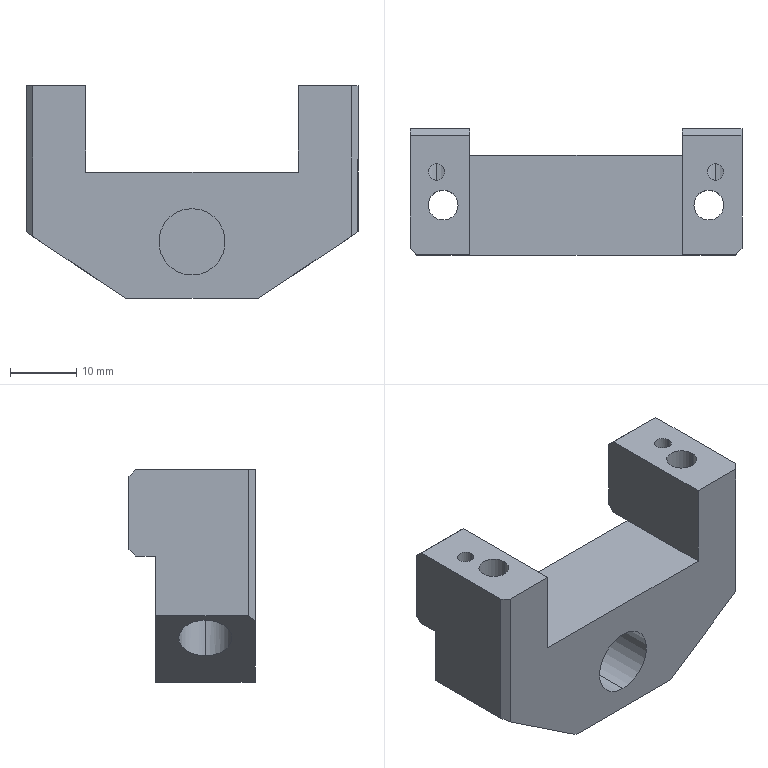Part | SolidWorks | features ICE 5, Chamfer 3, 3DProfileFeature 2, HoleWzd 2, Extrusion 1 | 1 solid | 45 faces | box 50 x 19 x 32 mm | volume 14007 mm3 | plane 27 | cylinder 18 | commonest cylinder face diameters 2.5 x4 4.5 x4 6 x4 8 x4 10 x2
STEP:
#1=CARTESIAN_POINT('',(0.,8.2,-2.5));
#2=VERTEX_POINT('',#1);
#3=CARTESIAN_POINT('',(0.,8.2,-12.5));
#4=VERTEX_POINT('',#3);
#5=CARTESIAN_POINT('',(0.,8.2,-7.5));
#6=DIRECTION('',(0.,-1.,0.));
#7=DIRECTION('',(0.,0.,-1.));
#8=AXIS2_PLACEMENT_3D('',#5,#6,#7);
#9=CIRCLE('',#8,5.);
#10=EDGE_CURVE('',#2,#4,#9,.T.);
#11=ORIENTED_EDGE('',*,*,#10,.F.);
#12=CARTESIAN_POINT('',(0.,0.,-2.5));
#13=VERTEX_POINT('',#12);
#14=CARTESIAN_POINT('',(0.,8.2,-2.5));
#15=DIRECTION('',(0.,-1.,0.));
#16=VECTOR('',#15,1000.);
#17=LINE('',#14,#16);
#18=EDGE_CURVE('',#2,#13,#17,.T.);
#19=ORIENTED_EDGE('',*,*,#18,.T.);
#20=CARTESIAN_POINT('',(0.,0.,-12.5));
#21=VERTEX_POINT('',#20);
#22=CARTESIAN_POINT('',(0.,0.,-7.5));
#23=DIRECTION('',(0.,-1.,0.));
#24=DIRECTION('',(0.,0.,-1.));
#25=AXIS2_PLACEMENT_3D('',#22,#23,#24);
#26=CIRCLE('',#25,5.);
#27=EDGE_CURVE('',#13,#21,#26,.T.);
#28=ORIENTED_EDGE('',*,*,#27,.T.);
#29=CARTESIAN_POINT('',(0.,8.2,-12.5));
#30=DIRECTION('',(0.,-1.,0.));
#31=VECTOR('',#30,1000.);
#32=LINE('',#29,#31);
#33=EDGE_CURVE('',#4,#21,#32,.T.);
#34=ORIENTED_EDGE('',*,*,#33,.F.);
#35=EDGE_LOOP('',(#11,#19,#28,#34));
#36=FACE_OUTER_BOUND('',#35,.T.);
#37=CARTESIAN_POINT('',(0.,8.2,-7.5));
#38=DIRECTION('',(0.,-1.,0.));
#39=DIRECTION('',(0.,0.,-1.));
#40=AXIS2_PLACEMENT_3D('',#37,#38,#39);
#41=CYLINDRICAL_SURFACE('',#40,5.);
#42=ADVANCED_FACE('',(#36),#41,.F.);
#43=CARTESIAN_POINT('',(19.75,12.5,10.727));
#44=VERTEX_POINT('',#43);
#45=CARTESIAN_POINT('',(21.,11.25,11.));
#46=VERTEX_POINT('',#45);
#47=CARTESIAN_POINT('',(19.75,12.5,10.727));
#48=CARTESIAN_POINT('',(19.75,12.335,10.727));
#49=CARTESIAN_POINT('',(19.784,12.169,10.743));
#50=CARTESIAN_POINT('',(19.909,11.868,10.795));
#51=CARTESIAN_POINT('',(20.001,11.731,10.831));
#52=CARTESIAN_POINT('',(20.23,11.502,10.902));
#53=CARTESIAN_POINT('',(20.366,11.41,10.936));
#54=CARTESIAN_POINT('',(20.67,11.283,10.986));
#55=CARTESIAN_POINT('',(20.833,11.25,11.));
#56=CARTESIAN_POINT('',(21.,11.25,11.));
#57=B_SPLINE_CURVE_WITH_KNOTS('',3,(#47,#48,#49,#50,#51,#52,#53,#54,#55,#56),.UNSPECIFIED.,.F.,.F.,(4,2,2,2,4),(0.005929,0.006423,0.006917,0.00741,0.007904),.UNSPECIFIED.);
#58=EDGE_CURVE('',#44,#46,#57,.T.);
#59=ORIENTED_EDGE('',*,*,#58,.F.);
#60=CARTESIAN_POINT('',(19.75,12.5,16.));
#61=VERTEX_POINT('',#60);
#62=CARTESIAN_POINT('',(19.75,12.5,16.));
#63=DIRECTION('',(0.,0.,1.));
#64=VECTOR('',#63,1000.);
#65=LINE('',#62,#64);
#66=EDGE_CURVE('',#44,#61,#65,.T.);
#67=ORIENTED_EDGE('',*,*,#66,.T.);
#68=CARTESIAN_POINT('',(22.25,12.5,16.));
#69=VERTEX_POINT('',#68);
#70=CARTESIAN_POINT('',(21.,12.5,16.));
#71=DIRECTION('',(0.,0.,1.));
#72=DIRECTION('',(1.,0.,0.));
#73=AXIS2_PLACEMENT_3D('',#70,#71,#72);
#74=CIRCLE('',#73,1.25);
#75=EDGE_CURVE('',#61,#69,#74,.T.);
#76=ORIENTED_EDGE('',*,*,#75,.T.);
#77=CARTESIAN_POINT('',(22.25,12.5,10.727));
#78=VERTEX_POINT('',#77);
#79=CARTESIAN_POINT('',(22.25,12.5,16.));
#80=DIRECTION('',(0.,0.,1.));
#81=VECTOR('',#80,1000.);
#82=LINE('',#79,#81);
#83=EDGE_CURVE('',#78,#69,#82,.T.);
#84=ORIENTED_EDGE('',*,*,#83,.F.);
#85=CARTESIAN_POINT('',(21.,11.25,11.));
#86=CARTESIAN_POINT('',(21.084,11.25,11.));
#87=CARTESIAN_POINT('',(21.166,11.258,10.997));
#88=CARTESIAN_POINT('',(21.327,11.291,10.983));
#89=CARTESIAN_POINT('',(21.407,11.315,10.973));
#90=CARTESIAN_POINT('',(21.634,11.41,10.936));
#91=CARTESIAN_POINT('',(21.771,11.503,10.902));
#92=CARTESIAN_POINT('',(21.999,11.731,10.831));
#93=CARTESIAN_POINT('',(22.091,11.869,10.795));
#94=CARTESIAN_POINT('',(22.216,12.169,10.743));
#95=CARTESIAN_POINT('',(22.25,12.335,10.727));
#96=CARTESIAN_POINT('',(22.25,12.5,10.727));
#97=B_SPLINE_CURVE_WITH_KNOTS('',3,(#85,#86,#87,#88,#89,#90,#91,#92,#93,#94,#95,#96),.UNSPECIFIED.,.F.,.F.,(4,2,2,2,2,4),(0.,0.0002472,0.0004944,0.0009888,0.001483,0.001978),.UNSPECIFIED.);
#98=EDGE_CURVE('',#46,#78,#97,.T.);
#99=ORIENTED_EDGE('',*,*,#98,.F.);
#100=EDGE_LOOP('',(#59,#67,#76,#84,#99));
#101=FACE_OUTER_BOUND('',#100,.T.);
#102=CARTESIAN_POINT('',(21.,12.5,16.));
#103=DIRECTION('',(0.,0.,1.));
#104=DIRECTION('',(1.,0.,0.));
#105=AXIS2_PLACEMENT_3D('',#102,#103,#104);
#106=CYLINDRICAL_SURFACE('',#105,1.25);
#107=ADVANCED_FACE('',(#101),#106,.F.);
#108=CARTESIAN_POINT('',(-22.25,12.5,10.727));
#109=VERTEX_POINT('',#108);
#110=CARTESIAN_POINT('',(-21.,11.25,11.));
#111=VERTEX_POINT('',#110);
#112=CARTESIAN_POINT('',(-22.25,12.5,10.727));
#113=CARTESIAN_POINT('',(-22.25,12.335,10.727));
#114=CARTESIAN_POINT('',(-22.216,12.169,10.743));
#115=CARTESIAN_POINT('',(-22.091,11.868,10.795));
#116=CARTESIAN_POINT('',(-21.999,11.731,10.831));
#117=CARTESIAN_POINT('',(-21.77,11.502,10.902));
#118=CARTESIAN_POINT('',(-21.634,11.41,10.936));
#119=CARTESIAN_POINT('',(-21.33,11.283,10.986));
#120=CARTESIAN_POINT('',(-21.167,11.25,11.));
#121=CARTESIAN_POINT('',(-21.,11.25,11.));
#122=B_SPLINE_CURVE_WITH_KNOTS('',3,(#112,#113,#114,#115,#116,#117,#118,#119,#120,#121),.UNSPECIFIED.,.F.,.F.,(4,2,2,2,4),(0.005929,0.006423,0.006917,0.00741,0.007904),.UNSPECIFIED.);
#123=EDGE_CURVE('',#109,#111,#122,.T.);
#124=ORIENTED_EDGE('',*,*,#123,.F.);
#125=CARTESIAN_POINT('',(-22.25,12.5,16.));
#126=VERTEX_POINT('',#125);
#127=CARTESIAN_POINT('',(-22.25,12.5,16.));
#128=DIRECTION('',(0.,0.,1.));
#129=VECTOR('',#128,1000.);
#130=LINE('',#127,#129);
#131=EDGE_CURVE('',#109,#126,#130,.T.);
#132=ORIENTED_EDGE('',*,*,#131,.T.);
#133=CARTESIAN_POINT('',(-19.75,12.5,16.));
#134=VERTEX_POINT('',#133);
#135=CARTESIAN_POINT('',(-21.,12.5,16.));
#136=DIRECTION('',(0.,0.,1.));
#137=DIRECTION('',(1.,0.,0.));
#138=AXIS2_PLACEMENT_3D('',#135,#136,#137);
#139=CIRCLE('',#138,1.25);
#140=EDGE_CURVE('',#126,#134,#139,.T.);
#141=ORIENTED_EDGE('',*,*,#140,.T.);
#142=CARTESIAN_POINT('',(-19.75,12.5,10.727));
#143=VERTEX_POINT('',#142);
#144=CARTESIAN_POINT('',(-19.75,12.5,16.));
#145=DIRECTION('',(0.,0.,1.));
#146=VECTOR('',#145,1000.);
#147=LINE('',#144,#146);
#148=EDGE_CURVE('',#143,#134,#147,.T.);
#149=ORIENTED_EDGE('',*,*,#148,.F.);
#150=CARTESIAN_POINT('',(-21.,11.25,11.));
#151=CARTESIAN_POINT('',(-20.916,11.25,11.));
#152=CARTESIAN_POINT('',(-20.834,11.258,10.997));
#153=CARTESIAN_POINT('',(-20.673,11.291,10.983));
#154=CARTESIAN_POINT('',(-20.593,11.315,10.973));
#155=CARTESIAN_POINT('',(-20.366,11.41,10.936));
#156=CARTESIAN_POINT('',(-20.229,11.503,10.902));
#157=CARTESIAN_POINT('',(-20.001,11.731,10.831));
#158=CARTESIAN_POINT('',(-19.909,11.869,10.795));
#159=CARTESIAN_POINT('',(-19.784,12.169,10.743));
#160=CARTESIAN_POINT('',(-19.75,12.335,10.727));
#161=CARTESIAN_POINT('',(-19.75,12.5,10.727));
#162=B_SPLINE_CURVE_WITH_KNOTS('',3,(#150,#151,#152,#153,#154,#155,#156,#157,#158,#159,#160,#161),.UNSPECIFIED.,.F.,.F.,(4,2,2,2,2,4),(0.,0.0002472,0.0004944,0.0009888,0.001483,0.001978),.UNSPECIFIED.);
#163=EDGE_CURVE('',#111,#143,#162,.T.);
#164=ORIENTED_EDGE('',*,*,#163,.F.);
#165=EDGE_LOOP('',(#124,#132,#141,#149,#164));
#166=FACE_OUTER_BOUND('',#165,.T.);
#167=CARTESIAN_POINT('',(-21.,12.5,16.));
#168=DIRECTION('',(0.,0.,1.));
#169=DIRECTION('',(1.,0.,0.));
#170=AXIS2_PLACEMENT_3D('',#167,#168,#169);
#171=CYLINDRICAL_SURFACE('',#170,1.25);
#172=ADVANCED_FACE('',(#166),#171,.F.);
#173=CARTESIAN_POINT('',(21.,10.8,5.));
#174=VERTEX_POINT('',#173);
#175=CARTESIAN_POINT('',(21.,10.8,11.));
#176=VERTEX_POINT('',#175);
#177=CARTESIAN_POINT('',(21.,10.8,8.));
#178=DIRECTION('',(0.,1.,0.));
#179=DIRECTION('',(0.,0.,1.));
#180=AXIS2_PLACEMENT_3D('',#177,#178,#179);
#181=CIRCLE('',#180,3.);
#182=EDGE_CURVE('',#174,#176,#181,.T.);
#183=ORIENTED_EDGE('',*,*,#182,.F.);
#184=CARTESIAN_POINT('',(21.,19.,5.));
#185=VERTEX_POINT('',#184);
#186=CARTESIAN_POINT('',(21.,10.8,5.));
#187=DIRECTION('',(0.,1.,0.));
#188=VECTOR('',#187,1000.);
#189=LINE('',#186,#188);
#190=EDGE_CURVE('',#174,#185,#189,.T.);
#191=ORIENTED_EDGE('',*,*,#190,.T.);
#192=CARTESIAN_POINT('',(21.,19.,11.));
#193=VERTEX_POINT('',#192);
#194=CARTESIAN_POINT('',(21.,19.,8.));
#195=DIRECTION('',(0.,1.,0.));
#196=DIRECTION('',(0.,0.,1.));
#197=AXIS2_PLACEMENT_3D('',#194,#195,#196);
#198=CIRCLE('',#197,3.);
#199=EDGE_CURVE('',#185,#193,#198,.T.);
#200=ORIENTED_EDGE('',*,*,#199,.T.);
#201=CARTESIAN_POINT('',(21.,13.75,11.));
#202=VERTEX_POINT('',#201);
#203=CARTESIAN_POINT('',(21.,10.8,11.));
#204=DIRECTION('',(0.,1.,0.));
#205=VECTOR('',#204,1000.);
#206=LINE('',#203,#205);
#207=EDGE_CURVE('',#202,#193,#206,.T.);
#208=ORIENTED_EDGE('',*,*,#207,.F.);
#209=CARTESIAN_POINT('',(21.,13.75,11.));
#210=CARTESIAN_POINT('',(20.835,13.75,11.));
#211=CARTESIAN_POINT('',(20.67,13.717,10.986));
#212=CARTESIAN_POINT('',(20.367,13.59,10.936));
#213=CARTESIAN_POINT('',(20.23,13.498,10.902));
#214=CARTESIAN_POINT('',(20.058,13.325,10.849));
#215=CARTESIAN_POINT('',(20.007,13.263,10.831));
#216=CARTESIAN_POINT('',(19.917,13.129,10.798));
#217=CARTESIAN_POINT('',(19.878,13.056,10.782));
#218=CARTESIAN_POINT('',(19.815,12.906,10.756));
#219=CARTESIAN_POINT('',(19.791,12.828,10.746));
#220=CARTESIAN_POINT('',(19.758,12.666,10.731));
#221=CARTESIAN_POINT('',(19.75,12.582,10.727));
#222=CARTESIAN_POINT('',(19.75,12.5,10.727));
#223=B_SPLINE_CURVE_WITH_KNOTS('',3,(#209,#210,#211,#212,#213,#214,#215,#216,#217,#218,#219,#220,#221,#222),.UNSPECIFIED.,.F.,.F.,(4,2,2,2,2,2,4),(0.003954,0.004448,0.004941,0.005188,0.005435,0.005682,0.005929),.UNSPECIFIED.);
#224=EDGE_CURVE('',#202,#44,#223,.T.);
#225=ORIENTED_EDGE('',*,*,#224,.T.);
#226=ORIENTED_EDGE('',*,*,#58,.T.);
#227=CARTESIAN_POINT('',(21.,10.8,11.));
#228=DIRECTION('',(0.,1.,0.));
#229=VECTOR('',#228,1000.);
#230=LINE('',#227,#229);
#231=EDGE_CURVE('',#176,#46,#230,.T.);
#232=ORIENTED_EDGE('',*,*,#231,.F.);
#233=EDGE_LOOP('',(#183,#191,#200,#208,#225,#226,#232));
#234=FACE_OUTER_BOUND('',#233,.T.);
#235=CARTESIAN_POINT('',(21.,10.8,8.));
#236=DIRECTION('',(0.,1.,0.));
#237=DIRECTION('',(0.,0.,1.));
#238=AXIS2_PLACEMENT_3D('',#235,#236,#237);
#239=CYLINDRICAL_SURFACE('',#238,3.);
#240=ADVANCED_FACE('',(#234),#239,.F.);
#241=CARTESIAN_POINT('',(-21.,10.8,5.));
#242=VERTEX_POINT('',#241);
#243=CARTESIAN_POINT('',(-21.,10.8,11.));
#244=VERTEX_POINT('',#243);
#245=CARTESIAN_POINT('',(-21.,10.8,8.));
#246=DIRECTION('',(0.,1.,0.));
#247=DIRECTION('',(0.,0.,1.));
#248=AXIS2_PLACEMENT_3D('',#245,#246,#247);
#249=CIRCLE('',#248,3.);
#250=EDGE_CURVE('',#242,#244,#249,.T.);
#251=ORIENTED_EDGE('',*,*,#250,.F.);
#252=CARTESIAN_POINT('',(-21.,19.,5.));
#253=VERTEX_POINT('',#252);
#254=CARTESIAN_POINT('',(-21.,10.8,5.));
#255=DIRECTION('',(0.,1.,0.));
#256=VECTOR('',#255,1000.);
#257=LINE('',#254,#256);
#258=EDGE_CURVE('',#242,#253,#257,.T.);
#259=ORIENTED_EDGE('',*,*,#258,.T.);
#260=CARTESIAN_POINT('',(-21.,19.,11.));
#261=VERTEX_POINT('',#260);
#262=CARTESIAN_POINT('',(-21.,19.,8.));
#263=DIRECTION('',(0.,1.,0.));
#264=DIRECTION('',(0.,0.,1.));
#265=AXIS2_PLACEMENT_3D('',#262,#263,#264);
#266=CIRCLE('',#265,3.);
#267=EDGE_CURVE('',#253,#261,#266,.T.);
#268=ORIENTED_EDGE('',*,*,#267,.T.);
#269=CARTESIAN_POINT('',(-21.,13.75,11.));
#270=VERTEX_POINT('',#269);
#271=CARTESIAN_POINT('',(-21.,10.8,11.));
#272=DIRECTION('',(0.,1.,0.));
#273=VECTOR('',#272,1000.);
#274=LINE('',#271,#273);
#275=EDGE_CURVE('',#270,#261,#274,.T.);
#276=ORIENTED_EDGE('',*,*,#275,.F.);
#277=CARTESIAN_POINT('',(-21.,13.75,11.));
#278=CARTESIAN_POINT('',(-21.165,13.75,11.));
#279=CARTESIAN_POINT('',(-21.33,13.717,10.986));
#280=CARTESIAN_POINT('',(-21.633,13.59,10.936));
#281=CARTESIAN_POINT('',(-21.77,13.498,10.902));
#282=CARTESIAN_POINT('',(-21.942,13.325,10.849));
#283=CARTESIAN_POINT('',(-21.993,13.263,10.831));
#284=CARTESIAN_POINT('',(-22.083,13.129,10.798));
#285=CARTESIAN_POINT('',(-22.122,13.056,10.782));
#286=CARTESIAN_POINT('',(-22.185,12.906,10.756));
#287=CARTESIAN_POINT('',(-22.209,12.828,10.746));
#288=CARTESIAN_POINT('',(-22.242,12.666,10.731));
#289=CARTESIAN_POINT('',(-22.25,12.582,10.727));
#290=CARTESIAN_POINT('',(-22.25,12.5,10.727));
#291=B_SPLINE_CURVE_WITH_KNOTS('',3,(#277,#278,#279,#280,#281,#282,#283,#284,#285,#286,#287,#288,#289,#290),.UNSPECIFIED.,.F.,.F.,(4,2,2,2,2,2,4),(0.003954,0.004448,0.004941,0.005188,0.005435,0.005682,0.005929),.UNSPECIFIED.);
#292=EDGE_CURVE('',#270,#109,#291,.T.);
#293=ORIENTED_EDGE('',*,*,#292,.T.);
#294=ORIENTED_EDGE('',*,*,#123,.T.);
#295=CARTESIAN_POINT('',(-21.,10.8,11.));
#296=DIRECTION('',(0.,1.,0.));
#297=VECTOR('',#296,1000.);
#298=LINE('',#295,#297);
#299=EDGE_CURVE('',#244,#111,#298,.T.);
#300=ORIENTED_EDGE('',*,*,#299,.F.);
#301=EDGE_LOOP('',(#251,#259,#268,#276,#293,#294,#300));
#302=FACE_OUTER_BOUND('',#301,.T.);
#303=CARTESIAN_POINT('',(-21.,10.8,8.));
#304=DIRECTION('',(0.,1.,0.));
#305=DIRECTION('',(0.,0.,1.));
#306=AXIS2_PLACEMENT_3D('',#303,#304,#305);
#307=CYLINDRICAL_SURFACE('',#306,3.);
#308=ADVANCED_FACE('',(#302),#307,.F.);
#309=CARTESIAN_POINT('',(-16.,7.5,-3.));
#310=VERTEX_POINT('',#309);
#311=CARTESIAN_POINT('',(-24.,7.5,-3.));
#312=VERTEX_POINT('',#311);
#313=CARTESIAN_POINT('',(-20.,7.5,-3.));
#314=DIRECTION('',(0.,0.,-1.));
#315=DIRECTION('',(-1.,0.,0.));
#316=AXIS2_PLACEMENT_3D('',#313,#314,#315);
#317=CIRCLE('',#316,4.);
#318=EDGE_CURVE('',#310,#312,#317,.T.);
#319=ORIENTED_EDGE('',*,*,#318,.F.);
#320=CARTESIAN_POINT('',(-16.,7.5,-12.));
#321=VERTEX_POINT('',#320);
#322=CARTESIAN_POINT('',(-16.,7.5,-3.));
#323=DIRECTION('',(0.,0.,-1.));
#324=VECTOR('',#323,1000.);
#325=LINE('',#322,#324);
#326=EDGE_CURVE('',#310,#321,#325,.T.);
#327=ORIENTED_EDGE('',*,*,#326,.T.);
#328=CARTESIAN_POINT('',(-24.,7.5,-6.667));
#329=VERTEX_POINT('',#328);
#330=CARTESIAN_POINT('',(-16.,7.5,-12.));
#331=CARTESIAN_POINT('',(-16.,-0.5,-12.));
#332=CARTESIAN_POINT('',(-24.,-0.5,-6.667));
#333=CARTESIAN_POINT('',(-24.,7.5,-6.667));
#334=(BOUNDED_CURVE()B_SPLINE_CURVE(3,(#330,#331,#332,#333),.UNSPECIFIED.,.F.,.F.)B_SPLINE_CURVE_WITH_KNOTS((4,4),(0.,3.142),.UNSPECIFIED.)CURVE()GEOMETRIC_REPRESENTATION_ITEM()RATIONAL_B_SPLINE_CURVE((1.,0.3333,0.3333,1.))REPRESENTATION_ITEM(''));
#335=EDGE_CURVE('',#321,#329,#334,.T.);
#336=ORIENTED_EDGE('',*,*,#335,.T.);
#337=CARTESIAN_POINT('',(-24.,7.5,-3.));
#338=DIRECTION('',(0.,0.,-1.));
#339=VECTOR('',#338,1000.);
#340=LINE('',#337,#339);
#341=EDGE_CURVE('',#312,#329,#340,.T.);
#342=ORIENTED_EDGE('',*,*,#341,.F.);
#343=EDGE_LOOP('',(#319,#327,#336,#342));
#344=FACE_OUTER_BOUND('',#343,.T.);
#345=CARTESIAN_POINT('',(-20.,7.5,-3.));
#346=DIRECTION('',(0.,0.,-1.));
#347=DIRECTION('',(-1.,0.,0.));
#348=AXIS2_PLACEMENT_3D('',#345,#346,#347);
#349=CYLINDRICAL_SURFACE('',#348,4.);
#350=ADVANCED_FACE('',(#344),#349,.F.);
#351=CARTESIAN_POINT('',(24.,7.5,-3.));
#352=VERTEX_POINT('',#351);
#353=CARTESIAN_POINT('',(16.,7.5,-3.));
#354=VERTEX_POINT('',#353);
#355=CARTESIAN_POINT('',(20.,7.5,-3.));
#356=DIRECTION('',(0.,0.,-1.));
#357=DIRECTION('',(-1.,0.,0.));
#358=AXIS2_PLACEMENT_3D('',#355,#356,#357);
#359=CIRCLE('',#358,4.);
#360=EDGE_CURVE('',#352,#354,#359,.T.);
#361=ORIENTED_EDGE('',*,*,#360,.F.);
#362=CARTESIAN_POINT('',(24.,7.5,-6.667));
#363=VERTEX_POINT('',#362);
#364=CARTESIAN_POINT('',(24.,7.5,-3.));
#365=DIRECTION('',(0.,0.,-1.));
#366=VECTOR('',#365,1000.);
#367=LINE('',#364,#366);
#368=EDGE_CURVE('',#352,#363,#367,.T.);
#369=ORIENTED_EDGE('',*,*,#368,.T.);
#370=CARTESIAN_POINT('',(16.,7.5,-12.));
#371=VERTEX_POINT('',#370);
#372=CARTESIAN_POINT('',(24.,7.5,-6.667));
#373=CARTESIAN_POINT('',(24.,-0.5,-6.667));
#374=CARTESIAN_POINT('',(16.,-0.5,-12.));
#375=CARTESIAN_POINT('',(16.,7.5,-12.));
#376=(BOUNDED_CURVE()B_SPLINE_CURVE(3,(#372,#373,#374,#375),.UNSPECIFIED.,.F.,.F.)B_SPLINE_CURVE_WITH_KNOTS((4,4),(3.142,6.283),.UNSPECIFIED.)CURVE()GEOMETRIC_REPRESENTATION_ITEM()RATIONAL_B_SPLINE_CURVE((1.,0.3333,0.3333,1.))REPRESENTATION_ITEM(''));
#377=EDGE_CURVE('',#363,#371,#376,.T.);
#378=ORIENTED_EDGE('',*,*,#377,.T.);
#379=CARTESIAN_POINT('',(16.,7.5,-3.));
#380=DIRECTION('',(0.,0.,-1.));
#381=VECTOR('',#380,1000.);
#382=LINE('',#379,#381);
#383=EDGE_CURVE('',#354,#371,#382,.T.);
#384=ORIENTED_EDGE('',*,*,#383,.F.);
#385=EDGE_LOOP('',(#361,#369,#378,#384));
#386=FACE_OUTER_BOUND('',#385,.T.);
#387=CARTESIAN_POINT('',(20.,7.5,-3.));
#388=DIRECTION('',(0.,0.,-1.));
#389=DIRECTION('',(-1.,0.,0.));
#390=AXIS2_PLACEMENT_3D('',#387,#388,#389);
#391=CYLINDRICAL_SURFACE('',#390,4.);
#392=ADVANCED_FACE('',(#386),#391,.F.);
#393=CARTESIAN_POINT('',(22.25,7.5,16.));
#394=VERTEX_POINT('',#393);
#395=CARTESIAN_POINT('',(17.75,7.5,16.));
#396=VERTEX_POINT('',#395);
#397=CARTESIAN_POINT('',(20.,7.5,16.));
#398=DIRECTION('',(0.,0.,-1.));
#399=DIRECTION('',(-1.,0.,0.));
#400=AXIS2_PLACEMENT_3D('',#397,#398,#399);
#401=CIRCLE('',#400,2.25);
#402=EDGE_CURVE('',#394,#396,#401,.T.);
#403=ORIENTED_EDGE('',*,*,#402,.F.);
#404=CARTESIAN_POINT('',(22.25,7.5,-3.));
#405=VERTEX_POINT('',#404);
#406=CARTESIAN_POINT('',(22.25,7.5,20.));
#407=DIRECTION('',(0.,0.,-1.));
#408=VECTOR('',#407,1000.);
#409=LINE('',#406,#408);
#410=EDGE_CURVE('',#394,#405,#409,.T.);
#411=ORIENTED_EDGE('',*,*,#410,.T.);
#412=CARTESIAN_POINT('',(17.75,7.5,-3.));
#413=VERTEX_POINT('',#412);
#414=CARTESIAN_POINT('',(20.,7.5,-3.));
#415=DIRECTION('',(0.,0.,1.));
#416=DIRECTION('',(-1.,0.,0.));
#417=AXIS2_PLACEMENT_3D('',#414,#415,#416);
#418=CIRCLE('',#417,2.25);
#419=EDGE_CURVE('',#413,#405,#418,.T.);
#420=ORIENTED_EDGE('',*,*,#419,.F.);
#421=CARTESIAN_POINT('',(17.75,7.5,20.));
#422=DIRECTION('',(0.,0.,-1.));
#423=VECTOR('',#422,1000.);
#424=LINE('',#421,#423);
#425=EDGE_CURVE('',#396,#413,#424,.T.);
#426=ORIENTED_EDGE('',*,*,#425,.F.);
#427=EDGE_LOOP('',(#403,#411,#420,#426));
#428=FACE_OUTER_BOUND('',#427,.T.);
#429=CARTESIAN_POINT('',(20.,7.5,20.));
#430=DIRECTION('',(0.,0.,-1.));
#431=DIRECTION('',(-1.,0.,0.));
#432=AXIS2_PLACEMENT_3D('',#429,#430,#431);
#433=CYLINDRICAL_SURFACE('',#432,2.25);
#434=ADVANCED_FACE('',(#428),#433,.F.);
#435=CARTESIAN_POINT('',(-17.75,7.5,16.));
#436=VERTEX_POINT('',#435);
#437=CARTESIAN_POINT('',(-22.25,7.5,16.));
#438=VERTEX_POINT('',#437);
#439=CARTESIAN_POINT('',(-20.,7.5,16.));
#440=DIRECTION('',(0.,0.,-1.));
#441=DIRECTION('',(-1.,0.,0.));
#442=AXIS2_PLACEMENT_3D('',#439,#440,#441);
#443=CIRCLE('',#442,2.25);
#444=EDGE_CURVE('',#436,#438,#443,.T.);
#445=ORIENTED_EDGE('',*,*,#444,.F.);
#446=CARTESIAN_POINT('',(-17.75,7.5,-3.));
#447=VERTEX_POINT('',#446);
#448=CARTESIAN_POINT('',(-17.75,7.5,20.));
#449=DIRECTION('',(0.,0.,-1.));
#450=VECTOR('',#449,1000.);
#451=LINE('',#448,#450);
#452=EDGE_CURVE('',#436,#447,#451,.T.);
#453=ORIENTED_EDGE('',*,*,#452,.T.);
#454=CARTESIAN_POINT('',(-22.25,7.5,-3.));
#455=VERTEX_POINT('',#454);
#456=CARTESIAN_POINT('',(-20.,7.5,-3.));
#457=DIRECTION('',(0.,0.,1.));
#458=DIRECTION('',(-1.,0.,0.));
#459=AXIS2_PLACEMENT_3D('',#456,#457,#458);
#460=CIRCLE('',#459,2.25);
#461=EDGE_CURVE('',#455,#447,#460,.T.);
#462=ORIENTED_EDGE('',*,*,#461,.F.);
#463=CARTESIAN_POINT('',(-22.25,7.5,20.));
#464=DIRECTION('',(0.,0.,-1.));
#465=VECTOR('',#464,1000.);
#466=LINE('',#463,#465);
#467=EDGE_CURVE('',#438,#455,#466,.T.);
#468=ORIENTED_EDGE('',*,*,#467,.F.);
#469=EDGE_LOOP('',(#445,#453,#462,#468));
#470=FACE_OUTER_BOUND('',#469,.T.);
#471=CARTESIAN_POINT('',(-20.,7.5,20.));
#472=DIRECTION('',(0.,0.,-1.));
#473=DIRECTION('',(-1.,0.,0.));
#474=AXIS2_PLACEMENT_3D('',#471,#472,#473);
#475=CYLINDRICAL_SURFACE('',#474,2.25);
#476=ADVANCED_FACE('',(#470),#475,.F.);
#477=CARTESIAN_POINT('',(25.,15.,3.));
#478=VERTEX_POINT('',#477);
#479=CARTESIAN_POINT('',(16.,15.,3.));
#480=VERTEX_POINT('',#479);
#481=CARTESIAN_POINT('',(16.,15.,3.));
#482=DIRECTION('',(-1.,0.,0.));
#483=VECTOR('',#482,1000.);
#484=LINE('',#481,#483);
#485=EDGE_CURVE('',#478,#480,#484,.T.);
#486=ORIENTED_EDGE('',*,*,#485,.F.);
#487=CARTESIAN_POINT('',(25.,15.,-6.));
#488=VERTEX_POINT('',#487);
#489=CARTESIAN_POINT('',(25.,15.,-16.));
#490=DIRECTION('',(0.,0.,-1.));
#491=VECTOR('',#490,1000.);
#492=LINE('',#489,#491);
#493=EDGE_CURVE('',#478,#488,#492,.T.);
#494=ORIENTED_EDGE('',*,*,#493,.T.);
#495=CARTESIAN_POINT('',(10.,15.,-16.));
#496=VERTEX_POINT('',#495);
#497=CARTESIAN_POINT('',(10.,15.,-16.));
#498=DIRECTION('',(-0.8321,0.,-0.5547));
#499=VECTOR('',#498,1000.);
#500=LINE('',#497,#499);
#501=EDGE_CURVE('',#488,#496,#500,.T.);
#502=ORIENTED_EDGE('',*,*,#501,.T.);
#503=CARTESIAN_POINT('',(-10.,15.,-16.));
#504=VERTEX_POINT('',#503);
#505=CARTESIAN_POINT('',(-25.,15.,-16.));
#506=DIRECTION('',(-1.,0.,0.));
#507=VECTOR('',#506,1000.);
#508=LINE('',#505,#507);
#509=EDGE_CURVE('',#496,#504,#508,.T.);
#510=ORIENTED_EDGE('',*,*,#509,.T.);
#511=CARTESIAN_POINT('',(-25.,15.,-6.));
#512=VERTEX_POINT('',#511);
#513=CARTESIAN_POINT('',(-25.,15.,-6.));
#514=DIRECTION('',(-0.8321,0.,0.5547));
#515=VECTOR('',#514,1000.);
#516=LINE('',#513,#515);
#517=EDGE_CURVE('',#504,#512,#516,.T.);
#518=ORIENTED_EDGE('',*,*,#517,.T.);
#519=CARTESIAN_POINT('',(-25.,15.,3.));
#520=VERTEX_POINT('',#519);
#521=CARTESIAN_POINT('',(-25.,15.,-16.));
#522=DIRECTION('',(0.,0.,1.));
#523=VECTOR('',#522,1000.);
#524=LINE('',#521,#523);
#525=EDGE_CURVE('',#512,#520,#524,.T.);
#526=ORIENTED_EDGE('',*,*,#525,.T.);
#527=CARTESIAN_POINT('',(-16.,15.,3.));
#528=VERTEX_POINT('',#527);
#529=CARTESIAN_POINT('',(-16.,15.,3.));
#530=DIRECTION('',(-1.,0.,0.));
#531=VECTOR('',#530,1000.);
#532=LINE('',#529,#531);
#533=EDGE_CURVE('',#528,#520,#532,.T.);
#534=ORIENTED_EDGE('',*,*,#533,.F.);
#535=CARTESIAN_POINT('',(-16.,15.,3.));
#536=DIRECTION('',(1.,0.,0.));
#537=VECTOR('',#536,1000.);
#538=LINE('',#535,#537);
#539=EDGE_CURVE('',#528,#480,#538,.T.);
#540=ORIENTED_EDGE('',*,*,#539,.T.);
#541=EDGE_LOOP('',(#486,#494,#502,#510,#518,#526,#534,#540));
#542=FACE_OUTER_BOUND('',#541,.T.);
#543=CARTESIAN_POINT('',(0.,15.,0.));
#544=DIRECTION('',(0.,-1.,0.));
#545=DIRECTION('',(0.,0.,-1.));
#546=AXIS2_PLACEMENT_3D('',#543,#544,#545);
#547=PLANE('',#546);
#548=ADVANCED_FACE('',(#542),#547,.F.);
#549=ORIENTED_EDGE('',*,*,#452,.F.);
#550=CARTESIAN_POINT('',(-20.,7.5,16.));
#551=DIRECTION('',(0.,0.,-1.));
#552=DIRECTION('',(-1.,0.,0.));
#553=AXIS2_PLACEMENT_3D('',#550,#551,#552);
#554=CIRCLE('',#553,2.25);
#555=EDGE_CURVE('',#438,#436,#554,.T.);
#556=ORIENTED_EDGE('',*,*,#555,.F.);
#557=ORIENTED_EDGE('',*,*,#467,.T.);
#558=CARTESIAN_POINT('',(-20.,7.5,-3.));
#559=DIRECTION('',(0.,0.,1.));
#560=DIRECTION('',(-1.,0.,0.));
#561=AXIS2_PLACEMENT_3D('',#558,#559,#560);
#562=CIRCLE('',#561,2.25);
#563=EDGE_CURVE('',#447,#455,#562,.T.);
#564=ORIENTED_EDGE('',*,*,#563,.F.);
#565=EDGE_LOOP('',(#549,#556,#557,#564));
#566=FACE_OUTER_BOUND('',#565,.T.);
#567=CARTESIAN_POINT('',(-20.,7.5,20.));
#568=DIRECTION('',(0.,0.,-1.));
#569=DIRECTION('',(-1.,0.,0.));
#570=AXIS2_PLACEMENT_3D('',#567,#568,#569);
#571=CYLINDRICAL_SURFACE('',#570,2.25);
#572=ADVANCED_FACE('',(#566),#571,.F.);
#573=ORIENTED_EDGE('',*,*,#410,.F.);
#574=CARTESIAN_POINT('',(20.,7.5,16.));
#575=DIRECTION('',(0.,0.,-1.));
#576=DIRECTION('',(-1.,0.,0.));
#577=AXIS2_PLACEMENT_3D('',#574,#575,#576);
#578=CIRCLE('',#577,2.25);
#579=EDGE_CURVE('',#396,#394,#578,.T.);
#580=ORIENTED_EDGE('',*,*,#579,.F.);
#581=ORIENTED_EDGE('',*,*,#425,.T.);
#582=CARTESIAN_POINT('',(20.,7.5,-3.));
#583=DIRECTION('',(0.,0.,1.));
#584=DIRECTION('',(-1.,0.,0.));
#585=AXIS2_PLACEMENT_3D('',#582,#583,#584);
#586=CIRCLE('',#585,2.25);
#587=EDGE_CURVE('',#405,#413,#586,.T.);
#588=ORIENTED_EDGE('',*,*,#587,.F.);
#589=EDGE_LOOP('',(#573,#580,#581,#588));
#590=FACE_OUTER_BOUND('',#589,.T.);
#591=CARTESIAN_POINT('',(20.,7.5,20.));
#592=DIRECTION('',(0.,0.,-1.));
#593=DIRECTION('',(-1.,0.,0.));
#594=AXIS2_PLACEMENT_3D('',#591,#592,#593);
#595=CYLINDRICAL_SURFACE('',#594,2.25);
#596=ADVANCED_FACE('',(#590),#595,.F.);
#597=CARTESIAN_POINT('',(21.,12.5,16.));
#598=DIRECTION('',(0.,0.,1.));
#599=DIRECTION('',(1.,0.,0.));
#600=AXIS2_PLACEMENT_3D('',#597,#598,#599);
#601=CIRCLE('',#600,1.25);
#602=EDGE_CURVE('',#69,#61,#601,.T.);
#603=ORIENTED_EDGE('',*,*,#602,.F.);
#604=ORIENTED_EDGE('',*,*,#75,.F.);
#605=EDGE_LOOP('',(#603,#604));
#606=FACE_BOUND('',#605,.T.);
#607=ORIENTED_EDGE('',*,*,#579,.T.);
#608=ORIENTED_EDGE('',*,*,#402,.T.);
#609=EDGE_LOOP('',(#607,#608));
#610=FACE_BOUND('',#609,.T.);
#611=CARTESIAN_POINT('',(25.,18.,16.));
#612=VERTEX_POINT('',#611);
#613=CARTESIAN_POINT('',(25.,1.,16.));
#614=VERTEX_POINT('',#613);
#615=CARTESIAN_POINT('',(25.,15.,16.));
#616=DIRECTION('',(0.,-1.,0.));
#617=VECTOR('',#616,1000.);
#618=LINE('',#615,#617);
#619=EDGE_CURVE('',#612,#614,#618,.T.);
#620=ORIENTED_EDGE('',*,*,#619,.F.);
#621=CARTESIAN_POINT('',(16.,18.,16.));
#622=VERTEX_POINT('',#621);
#623=CARTESIAN_POINT('',(16.,18.,16.));
#624=DIRECTION('',(-1.,0.,0.));
#625=VECTOR('',#624,1000.);
#626=LINE('',#623,#625);
#627=EDGE_CURVE('',#612,#622,#626,.T.);
#628=ORIENTED_EDGE('',*,*,#627,.T.);
#629=CARTESIAN_POINT('',(16.,0.,16.));
#630=VERTEX_POINT('',#629);
#631=CARTESIAN_POINT('',(16.,15.,16.));
#632=DIRECTION('',(0.,-1.,0.));
#633=VECTOR('',#632,1000.);
#634=LINE('',#631,#633);
#635=EDGE_CURVE('',#622,#630,#634,.T.);
#636=ORIENTED_EDGE('',*,*,#635,.T.);
#637=CARTESIAN_POINT('',(24.,0.,16.));
#638=VERTEX_POINT('',#637);
#639=CARTESIAN_POINT('',(16.,0.,16.));
#640=DIRECTION('',(1.,0.,0.));
#641=VECTOR('',#640,1000.);
#642=LINE('',#639,#641);
#643=EDGE_CURVE('',#630,#638,#642,.T.);
#644=ORIENTED_EDGE('',*,*,#643,.T.);
#645=CARTESIAN_POINT('',(25.,1.,16.));
#646=DIRECTION('',(0.7071,0.7071,0.));
#647=VECTOR('',#646,1000.);
#648=LINE('',#645,#647);
#649=EDGE_CURVE('',#638,#614,#648,.T.);
#650=ORIENTED_EDGE('',*,*,#649,.T.);
#651=EDGE_LOOP('',(#620,#628,#636,#644,#650));
#652=FACE_OUTER_BOUND('',#651,.T.);
#653=CARTESIAN_POINT('',(16.,15.,16.));
#654=DIRECTION('',(0.,0.,-1.));
#655=DIRECTION('',(-1.,0.,0.));
#656=AXIS2_PLACEMENT_3D('',#653,#654,#655);
#657=PLANE('',#656);
#658=ADVANCED_FACE('',(#606,#610,#652),#657,.F.);
#659=CARTESIAN_POINT('',(25.,18.,3.));
#660=VERTEX_POINT('',#659);
#661=CARTESIAN_POINT('',(25.,19.,3.));
#662=DIRECTION('',(0.,-1.,0.));
#663=VECTOR('',#662,1000.);
#664=LINE('',#661,#663);
#665=EDGE_CURVE('',#660,#478,#664,.T.);
#666=ORIENTED_EDGE('',*,*,#665,.F.);
#667=CARTESIAN_POINT('',(25.,19.,4.));
#668=VERTEX_POINT('',#667);
#669=CARTESIAN_POINT('',(25.,19.,4.));
#670=DIRECTION('',(0.,0.7071,0.7071));
#671=VECTOR('',#670,1000.);
#672=LINE('',#669,#671);
#673=EDGE_CURVE('',#660,#668,#672,.T.);
#674=ORIENTED_EDGE('',*,*,#673,.T.);
#675=CARTESIAN_POINT('',(25.,19.,15.));
#676=VERTEX_POINT('',#675);
#677=CARTESIAN_POINT('',(25.,19.,3.));
#678=DIRECTION('',(0.,0.,-1.));
#679=VECTOR('',#678,1000.);
#680=LINE('',#677,#679);
#681=EDGE_CURVE('',#676,#668,#680,.T.);
#682=ORIENTED_EDGE('',*,*,#681,.F.);
#683=CARTESIAN_POINT('',(25.,19.,15.));
#684=DIRECTION('',(0.,-0.7071,0.7071));
#685=VECTOR('',#684,1000.);
#686=LINE('',#683,#685);
#687=EDGE_CURVE('',#676,#612,#686,.T.);
#688=ORIENTED_EDGE('',*,*,#687,.T.);
#689=ORIENTED_EDGE('',*,*,#619,.T.);
#690=CARTESIAN_POINT('',(25.,1.,-6.));
#691=VERTEX_POINT('',#690);
#692=CARTESIAN_POINT('',(25.,1.,-6.));
#693=DIRECTION('',(0.,0.,-1.));
#694=VECTOR('',#693,1000.);
#695=LINE('',#692,#694);
#696=EDGE_CURVE('',#614,#691,#695,.T.);
#697=ORIENTED_EDGE('',*,*,#696,.T.);
#698=CARTESIAN_POINT('',(25.,15.,-6.));
#699=DIRECTION('',(0.,1.,0.));
#700=VECTOR('',#699,1000.);
#701=LINE('',#698,#700);
#702=EDGE_CURVE('',#691,#488,#701,.T.);
#703=ORIENTED_EDGE('',*,*,#702,.T.);
#704=ORIENTED_EDGE('',*,*,#493,.F.);
#705=EDGE_LOOP('',(#666,#674,#682,#688,#689,#697,#703,#704));
#706=FACE_OUTER_BOUND('',#705,.T.);
#707=CARTESIAN_POINT('',(25.,15.,-16.));
#708=DIRECTION('',(-1.,0.,0.));
#709=DIRECTION('',(0.,0.,1.));
#710=AXIS2_PLACEMENT_3D('',#707,#708,#709);
#711=PLANE('',#710);
#712=ADVANCED_FACE('',(#706),#711,.F.);
#713=CARTESIAN_POINT('',(10.,0.,-16.));
#714=VERTEX_POINT('',#713);
#715=CARTESIAN_POINT('',(-10.,0.,-16.));
#716=VERTEX_POINT('',#715);
#717=CARTESIAN_POINT('',(-25.,0.,-16.));
#718=DIRECTION('',(-1.,0.,0.));
#719=VECTOR('',#718,1000.);
#720=LINE('',#717,#719);
#721=EDGE_CURVE('',#714,#716,#720,.T.);
#722=ORIENTED_EDGE('',*,*,#721,.T.);
#723=CARTESIAN_POINT('',(-10.,15.,-16.));
#724=DIRECTION('',(0.,1.,0.));
#725=VECTOR('',#724,1000.);
#726=LINE('',#723,#725);
#727=EDGE_CURVE('',#716,#504,#726,.T.);
#728=ORIENTED_EDGE('',*,*,#727,.T.);
#729=ORIENTED_EDGE('',*,*,#509,.F.);
#730=CARTESIAN_POINT('',(10.,15.,-16.));
#731=DIRECTION('',(0.,-1.,0.));
#732=VECTOR('',#731,1000.);
#733=LINE('',#730,#732);
#734=EDGE_CURVE('',#496,#714,#733,.T.);
#735=ORIENTED_EDGE('',*,*,#734,.T.);
#736=EDGE_LOOP('',(#722,#728,#729,#735));
#737=FACE_OUTER_BOUND('',#736,.T.);
#738=CARTESIAN_POINT('',(-25.,15.,-16.));
#739=DIRECTION('',(0.,0.,1.));
#740=DIRECTION('',(1.,0.,0.));
#741=AXIS2_PLACEMENT_3D('',#738,#739,#740);
#742=PLANE('',#741);
#743=ADVANCED_FACE('',(#737),#742,.F.);
#744=CARTESIAN_POINT('',(-25.,19.,4.));
#745=VERTEX_POINT('',#744);
#746=CARTESIAN_POINT('',(-25.,19.,15.));
#747=VERTEX_POINT('',#746);
#748=CARTESIAN_POINT('',(-25.,19.,3.));
#749=DIRECTION('',(0.,0.,1.));
#750=VECTOR('',#749,1000.);
#751=LINE('',#748,#750);
#752=EDGE_CURVE('',#745,#747,#751,.T.);
#753=ORIENTED_EDGE('',*,*,#752,.F.);
#754=CARTESIAN_POINT('',(-25.,18.,3.));
#755=VERTEX_POINT('',#754);
#756=CARTESIAN_POINT('',(-25.,19.,4.));
#757=DIRECTION('',(0.,-0.7071,-0.7071));
#758=VECTOR('',#757,1000.);
#759=LINE('',#756,#758);
#760=EDGE_CURVE('',#745,#755,#759,.T.);
#761=ORIENTED_EDGE('',*,*,#760,.T.);
#762=CARTESIAN_POINT('',(-25.,19.,3.));
#763=DIRECTION('',(0.,-1.,0.));
#764=VECTOR('',#763,1000.);
#765=LINE('',#762,#764);
#766=EDGE_CURVE('',#755,#520,#765,.T.);
#767=ORIENTED_EDGE('',*,*,#766,.T.);
#768=ORIENTED_EDGE('',*,*,#525,.F.);
#769=CARTESIAN_POINT('',(-25.,1.,-6.));
#770=VERTEX_POINT('',#769);
#771=CARTESIAN_POINT('',(-25.,15.,-6.));
#772=DIRECTION('',(0.,-1.,0.));
#773=VECTOR('',#772,1000.);
#774=LINE('',#771,#773);
#775=EDGE_CURVE('',#512,#770,#774,.T.);
#776=ORIENTED_EDGE('',*,*,#775,.T.);
#777=CARTESIAN_POINT('',(-25.,1.,16.));
#778=VERTEX_POINT('',#777);
#779=CARTESIAN_POINT('',(-25.,1.,16.));
#780=DIRECTION('',(0.,0.,1.));
#781=VECTOR('',#780,1000.);
#782=LINE('',#779,#781);
#783=EDGE_CURVE('',#770,#778,#782,.T.);
#784=ORIENTED_EDGE('',*,*,#783,.T.);
#785=CARTESIAN_POINT('',(-25.,18.,16.));
#786=VERTEX_POINT('',#785);
#787=CARTESIAN_POINT('',(-25.,15.,16.));
#788=DIRECTION('',(0.,-1.,0.));
#789=VECTOR('',#788,1000.);
#790=LINE('',#787,#789);
#791=EDGE_CURVE('',#786,#778,#790,.T.);
#792=ORIENTED_EDGE('',*,*,#791,.F.);
#793=CARTESIAN_POINT('',(-25.,19.,15.));
#794=DIRECTION('',(0.,0.7071,-0.7071));
#795=VECTOR('',#794,1000.);
#796=LINE('',#793,#795);
#797=EDGE_CURVE('',#786,#747,#796,.T.);
#798=ORIENTED_EDGE('',*,*,#797,.T.);
#799=EDGE_LOOP('',(#753,#761,#767,#768,#776,#784,#792,#798));
#800=FACE_OUTER_BOUND('',#799,.T.);
#801=CARTESIAN_POINT('',(-25.,15.,-16.));
#802=DIRECTION('',(1.,0.,0.));
#803=DIRECTION('',(0.,0.,-1.));
#804=AXIS2_PLACEMENT_3D('',#801,#802,#803);
#805=PLANE('',#804);
#806=ADVANCED_FACE('',(#800),#805,.F.);
#807=CARTESIAN_POINT('',(-21.,12.5,16.));
#808=DIRECTION('',(0.,0.,1.));
#809=DIRECTION('',(1.,0.,0.));
#810=AXIS2_PLACEMENT_3D('',#807,#808,#809);
#811=CIRCLE('',#810,1.25);
#812=EDGE_CURVE('',#134,#126,#811,.T.);
#813=ORIENTED_EDGE('',*,*,#812,.F.);
#814=ORIENTED_EDGE('',*,*,#140,.F.);
#815=EDGE_LOOP('',(#813,#814));
#816=FACE_BOUND('',#815,.T.);
#817=ORIENTED_EDGE('',*,*,#555,.T.);
#818=ORIENTED_EDGE('',*,*,#444,.T.);
#819=EDGE_LOOP('',(#817,#818));
#820=FACE_BOUND('',#819,.T.);
#821=CARTESIAN_POINT('',(-16.,18.,16.));
#822=VERTEX_POINT('',#821);
#823=CARTESIAN_POINT('',(-16.,0.,16.));
#824=VERTEX_POINT('',#823);
#825=CARTESIAN_POINT('',(-16.,15.,16.));
#826=DIRECTION('',(0.,-1.,0.));
#827=VECTOR('',#826,1000.);
#828=LINE('',#825,#827);
#829=EDGE_CURVE('',#822,#824,#828,.T.);
#830=ORIENTED_EDGE('',*,*,#829,.F.);
#831=CARTESIAN_POINT('',(-25.,18.,16.));
#832=DIRECTION('',(-1.,0.,0.));
#833=VECTOR('',#832,1000.);
#834=LINE('',#831,#833);
#835=EDGE_CURVE('',#822,#786,#834,.T.);
#836=ORIENTED_EDGE('',*,*,#835,.T.);
#837=ORIENTED_EDGE('',*,*,#791,.T.);
#838=CARTESIAN_POINT('',(-24.,0.,16.));
#839=VERTEX_POINT('',#838);
#840=CARTESIAN_POINT('',(-25.,1.,16.));
#841=DIRECTION('',(0.7071,-0.7071,0.));
#842=VECTOR('',#841,1000.);
#843=LINE('',#840,#842);
#844=EDGE_CURVE('',#778,#839,#843,.T.);
#845=ORIENTED_EDGE('',*,*,#844,.T.);
#846=CARTESIAN_POINT('',(-25.,0.,16.));
#847=DIRECTION('',(1.,0.,0.));
#848=VECTOR('',#847,1000.);
#849=LINE('',#846,#848);
#850=EDGE_CURVE('',#839,#824,#849,.T.);
#851=ORIENTED_EDGE('',*,*,#850,.T.);
#852=EDGE_LOOP('',(#830,#836,#837,#845,#851));
#853=FACE_OUTER_BOUND('',#852,.T.);
#854=CARTESIAN_POINT('',(-25.,15.,16.));
#855=DIRECTION('',(0.,0.,-1.));
#856=DIRECTION('',(-1.,0.,0.));
#857=AXIS2_PLACEMENT_3D('',#854,#855,#856);
#858=PLANE('',#857);
#859=ADVANCED_FACE('',(#816,#820,#853),#858,.F.);
#860=CARTESIAN_POINT('',(-16.,18.,3.));
#861=VERTEX_POINT('',#860);
#862=CARTESIAN_POINT('',(-16.,19.,3.));
#863=DIRECTION('',(0.,-1.,0.));
#864=VECTOR('',#863,1000.);
#865=LINE('',#862,#864);
#866=EDGE_CURVE('',#861,#528,#865,.T.);
#867=ORIENTED_EDGE('',*,*,#866,.F.);
#868=CARTESIAN_POINT('',(-16.,19.,4.));
#869=VERTEX_POINT('',#868);
#870=CARTESIAN_POINT('',(-16.,19.,4.));
#871=DIRECTION('',(0.,0.7071,0.7071));
#872=VECTOR('',#871,1000.);
#873=LINE('',#870,#872);
#874=EDGE_CURVE('',#861,#869,#873,.T.);
#875=ORIENTED_EDGE('',*,*,#874,.T.);
#876=CARTESIAN_POINT('',(-16.,19.,15.));
#877=VERTEX_POINT('',#876);
#878=CARTESIAN_POINT('',(-16.,19.,3.));
#879=DIRECTION('',(0.,0.,-1.));
#880=VECTOR('',#879,1000.);
#881=LINE('',#878,#880);
#882=EDGE_CURVE('',#877,#869,#881,.T.);
#883=ORIENTED_EDGE('',*,*,#882,.F.);
#884=CARTESIAN_POINT('',(-16.,19.,15.));
#885=DIRECTION('',(0.,-0.7071,0.7071));
#886=VECTOR('',#885,1000.);
#887=LINE('',#884,#886);
#888=EDGE_CURVE('',#877,#822,#887,.T.);
#889=ORIENTED_EDGE('',*,*,#888,.T.);
#890=ORIENTED_EDGE('',*,*,#829,.T.);
#891=CARTESIAN_POINT('',(-16.,0.,3.));
#892=VERTEX_POINT('',#891);
#893=CARTESIAN_POINT('',(-16.,0.,3.));
#894=DIRECTION('',(0.,0.,-1.));
#895=VECTOR('',#894,1000.);
#896=LINE('',#893,#895);
#897=EDGE_CURVE('',#824,#892,#896,.T.);
#898=ORIENTED_EDGE('',*,*,#897,.T.);
#899=CARTESIAN_POINT('',(-16.,15.,3.));
#900=DIRECTION('',(0.,-1.,0.));
#901=VECTOR('',#900,1000.);
#902=LINE('',#899,#901);
#903=EDGE_CURVE('',#528,#892,#902,.T.);
#904=ORIENTED_EDGE('',*,*,#903,.F.);
#905=EDGE_LOOP('',(#867,#875,#883,#889,#890,#898,#904));
#906=FACE_OUTER_BOUND('',#905,.T.);
#907=CARTESIAN_POINT('',(-16.,15.,3.));
#908=DIRECTION('',(-1.,0.,0.));
#909=DIRECTION('',(0.,0.,1.));
#910=AXIS2_PLACEMENT_3D('',#907,#908,#909);
#911=PLANE('',#910);
#912=ADVANCED_FACE('',(#906),#911,.F.);
#913=CARTESIAN_POINT('',(16.,0.,3.));
#914=VERTEX_POINT('',#913);
#915=CARTESIAN_POINT('',(-16.,0.,3.));
#916=DIRECTION('',(1.,0.,0.));
#917=VECTOR('',#916,1000.);
#918=LINE('',#915,#917);
#919=EDGE_CURVE('',#892,#914,#918,.T.);
#920=ORIENTED_EDGE('',*,*,#919,.T.);
#921=CARTESIAN_POINT('',(16.,15.,3.));
#922=DIRECTION('',(0.,-1.,0.));
#923=VECTOR('',#922,1000.);
#924=LINE('',#921,#923);
#925=EDGE_CURVE('',#480,#914,#924,.T.);
#926=ORIENTED_EDGE('',*,*,#925,.F.);
#927=ORIENTED_EDGE('',*,*,#539,.F.);
#928=ORIENTED_EDGE('',*,*,#903,.T.);
#929=EDGE_LOOP('',(#920,#926,#927,#928));
#930=FACE_OUTER_BOUND('',#929,.T.);
#931=CARTESIAN_POINT('',(-16.,15.,3.));
#932=DIRECTION('',(0.,0.,-1.));
#933=DIRECTION('',(-1.,0.,0.));
#934=AXIS2_PLACEMENT_3D('',#931,#932,#933);
#935=PLANE('',#934);
#936=ADVANCED_FACE('',(#930),#935,.F.);
#937=CARTESIAN_POINT('',(16.,19.,4.));
#938=VERTEX_POINT('',#937);
#939=CARTESIAN_POINT('',(16.,19.,15.));
#940=VERTEX_POINT('',#939);
#941=CARTESIAN_POINT('',(16.,19.,3.));
#942=DIRECTION('',(0.,0.,1.));
#943=VECTOR('',#942,1000.);
#944=LINE('',#941,#943);
#945=EDGE_CURVE('',#938,#940,#944,.T.);
#946=ORIENTED_EDGE('',*,*,#945,.F.);
#947=CARTESIAN_POINT('',(16.,18.,3.));
#948=VERTEX_POINT('',#947);
#949=CARTESIAN_POINT('',(16.,19.,4.));
#950=DIRECTION('',(0.,-0.7071,-0.7071));
#951=VECTOR('',#950,1000.);
#952=LINE('',#949,#951);
#953=EDGE_CURVE('',#938,#948,#952,.T.);
#954=ORIENTED_EDGE('',*,*,#953,.T.);
#955=CARTESIAN_POINT('',(16.,19.,3.));
#956=DIRECTION('',(0.,-1.,0.));
#957=VECTOR('',#956,1000.);
#958=LINE('',#955,#957);
#959=EDGE_CURVE('',#948,#480,#958,.T.);
#960=ORIENTED_EDGE('',*,*,#959,.T.);
#961=ORIENTED_EDGE('',*,*,#925,.T.);
#962=CARTESIAN_POINT('',(16.,0.,3.));
#963=DIRECTION('',(0.,0.,1.));
#964=VECTOR('',#963,1000.);
#965=LINE('',#962,#964);
#966=EDGE_CURVE('',#914,#630,#965,.T.);
#967=ORIENTED_EDGE('',*,*,#966,.T.);
#968=ORIENTED_EDGE('',*,*,#635,.F.);
#969=CARTESIAN_POINT('',(16.,19.,15.));
#970=DIRECTION('',(0.,0.7071,-0.7071));
#971=VECTOR('',#970,1000.);
#972=LINE('',#969,#971);
#973=EDGE_CURVE('',#622,#940,#972,.T.);
#974=ORIENTED_EDGE('',*,*,#973,.T.);
#975=EDGE_LOOP('',(#946,#954,#960,#961,#967,#968,#974));
#976=FACE_OUTER_BOUND('',#975,.T.);
#977=CARTESIAN_POINT('',(16.,15.,3.));
#978=DIRECTION('',(1.,0.,0.));
#979=DIRECTION('',(0.,0.,-1.));
#980=AXIS2_PLACEMENT_3D('',#977,#978,#979);
#981=PLANE('',#980);
#982=ADVANCED_FACE('',(#976),#981,.F.);
#983=CARTESIAN_POINT('',(0.,0.,-7.5));
#984=DIRECTION('',(0.,-1.,0.));
#985=DIRECTION('',(0.,0.,-1.));
#986=AXIS2_PLACEMENT_3D('',#983,#984,#985);
#987=CIRCLE('',#986,5.);
#988=EDGE_CURVE('',#21,#13,#987,.T.);
#989=ORIENTED_EDGE('',*,*,#988,.F.);
#990=ORIENTED_EDGE('',*,*,#27,.F.);
#991=EDGE_LOOP('',(#989,#990));
#992=FACE_BOUND('',#991,.T.);
#993=ORIENTED_EDGE('',*,*,#850,.F.);
#994=CARTESIAN_POINT('',(-24.,0.,-6.667));
#995=VERTEX_POINT('',#994);
#996=CARTESIAN_POINT('',(-24.,0.,-6.));
#997=DIRECTION('',(0.,0.,-1.));
#998=VECTOR('',#997,1000.);
#999=LINE('',#996,#998);
#1000=EDGE_CURVE('',#839,#995,#999,.T.);
#1001=ORIENTED_EDGE('',*,*,#1000,.T.);
#1002=CARTESIAN_POINT('',(-10.462,0.,-15.692));
#1003=DIRECTION('',(0.8321,0.,-0.5547));
#1004=VECTOR('',#1003,1000.);
#1005=LINE('',#1002,#1004);
#1006=EDGE_CURVE('',#995,#716,#1005,.T.);
#1007=ORIENTED_EDGE('',*,*,#1006,.T.);
#1008=ORIENTED_EDGE('',*,*,#721,.F.);
#1009=CARTESIAN_POINT('',(24.,0.,-6.667));
#1010=VERTEX_POINT('',#1009);
#1011=CARTESIAN_POINT('',(10.462,0.,-15.692));
#1012=DIRECTION('',(0.8321,0.,0.5547));
#1013=VECTOR('',#1012,1000.);
#1014=LINE('',#1011,#1013);
#1015=EDGE_CURVE('',#714,#1010,#1014,.T.);
#1016=ORIENTED_EDGE('',*,*,#1015,.T.);
#1017=CARTESIAN_POINT('',(24.,0.,16.));
#1018=DIRECTION('',(0.,0.,1.));
#1019=VECTOR('',#1018,1000.);
#1020=LINE('',#1017,#1019);
#1021=EDGE_CURVE('',#1010,#638,#1020,.T.);
#1022=ORIENTED_EDGE('',*,*,#1021,.T.);
#1023=ORIENTED_EDGE('',*,*,#643,.F.);
#1024=ORIENTED_EDGE('',*,*,#966,.F.);
#1025=ORIENTED_EDGE('',*,*,#919,.F.);
#1026=ORIENTED_EDGE('',*,*,#897,.F.);
#1027=EDGE_LOOP('',(#993,#1001,#1007,#1008,#1016,#1022,#1023,#1024,#1025,#1026));
#1028=FACE_OUTER_BOUND('',#1027,.T.);
#1029=CARTESIAN_POINT('',(0.,0.,0.));
#1030=DIRECTION('',(0.,-1.,0.));
#1031=DIRECTION('',(0.,0.,-1.));
#1032=AXIS2_PLACEMENT_3D('',#1029,#1030,#1031);
#1033=PLANE('',#1032);
#1034=ADVANCED_FACE('',(#992,#1028),#1033,.T.);
#1035=CARTESIAN_POINT('',(16.,7.5,-12.));
#1036=CARTESIAN_POINT('',(16.,15.5,-12.));
#1037=CARTESIAN_POINT('',(24.,15.5,-6.667));
#1038=CARTESIAN_POINT('',(24.,7.5,-6.667));
#1039=(BOUNDED_CURVE()B_SPLINE_CURVE(3,(#1035,#1036,#1037,#1038),.UNSPECIFIED.,.F.,.F.)B_SPLINE_CURVE_WITH_KNOTS((4,4),(0.,3.142),.UNSPECIFIED.)CURVE()GEOMETRIC_REPRESENTATION_ITEM()RATIONAL_B_SPLINE_CURVE((1.,0.3333,0.3333,1.))REPRESENTATION_ITEM(''));
#1040=EDGE_CURVE('',#371,#363,#1039,.T.);
#1041=ORIENTED_EDGE('',*,*,#1040,.F.);
#1042=ORIENTED_EDGE('',*,*,#377,.F.);
#1043=EDGE_LOOP('',(#1041,#1042));
#1044=FACE_BOUND('',#1043,.T.);
#1045=ORIENTED_EDGE('',*,*,#702,.F.);
#1046=CARTESIAN_POINT('',(21.864,-2.136,-8.091));
#1047=DIRECTION('',(-0.6396,-0.6396,-0.4264));
#1048=VECTOR('',#1047,1000.);
#1049=LINE('',#1046,#1048);
#1050=EDGE_CURVE('',#691,#1010,#1049,.T.);
#1051=ORIENTED_EDGE('',*,*,#1050,.T.);
#1052=ORIENTED_EDGE('',*,*,#1015,.F.);
#1053=ORIENTED_EDGE('',*,*,#734,.F.);
#1054=ORIENTED_EDGE('',*,*,#501,.F.);
#1055=EDGE_LOOP('',(#1045,#1051,#1052,#1053,#1054));
#1056=FACE_OUTER_BOUND('',#1055,.T.);
#1057=CARTESIAN_POINT('',(10.,15.,-16.));
#1058=DIRECTION('',(-0.5547,0.,0.8321));
#1059=DIRECTION('',(0.,-1.,0.));
#1060=AXIS2_PLACEMENT_3D('',#1057,#1058,#1059);
#1061=PLANE('',#1060);
#1062=ADVANCED_FACE('',(#1044,#1056),#1061,.F.);
#1063=CARTESIAN_POINT('',(-24.,7.5,-6.667));
#1064=CARTESIAN_POINT('',(-24.,15.5,-6.667));
#1065=CARTESIAN_POINT('',(-16.,15.5,-12.));
#1066=CARTESIAN_POINT('',(-16.,7.5,-12.));
#1067=(BOUNDED_CURVE()B_SPLINE_CURVE(3,(#1063,#1064,#1065,#1066),.UNSPECIFIED.,.F.,.F.)B_SPLINE_CURVE_WITH_KNOTS((4,4),(3.142,6.283),.UNSPECIFIED.)CURVE()GEOMETRIC_REPRESENTATION_ITEM()RATIONAL_B_SPLINE_CURVE((1.,0.3333,0.3333,1.))REPRESENTATION_ITEM(''));
#1068=EDGE_CURVE('',#329,#321,#1067,.T.);
#1069=ORIENTED_EDGE('',*,*,#1068,.F.);
#1070=ORIENTED_EDGE('',*,*,#335,.F.);
#1071=EDGE_LOOP('',(#1069,#1070));
#1072=FACE_BOUND('',#1071,.T.);
#1073=ORIENTED_EDGE('',*,*,#1006,.F.);
#1074=CARTESIAN_POINT('',(-30.727,6.727,-2.182));
#1075=DIRECTION('',(-0.6396,0.6396,0.4264));
#1076=VECTOR('',#1075,1000.);
#1077=LINE('',#1074,#1076);
#1078=EDGE_CURVE('',#995,#770,#1077,.T.);
#1079=ORIENTED_EDGE('',*,*,#1078,.T.);
#1080=ORIENTED_EDGE('',*,*,#775,.F.);
#1081=ORIENTED_EDGE('',*,*,#517,.F.);
#1082=ORIENTED_EDGE('',*,*,#727,.F.);
#1083=EDGE_LOOP('',(#1073,#1079,#1080,#1081,#1082));
#1084=FACE_OUTER_BOUND('',#1083,.T.);
#1085=CARTESIAN_POINT('',(-25.,15.,-6.));
#1086=DIRECTION('',(0.5547,0.,0.8321));
#1087=DIRECTION('',(0.,-1.,0.));
#1088=AXIS2_PLACEMENT_3D('',#1085,#1086,#1087);
#1089=PLANE('',#1088);
#1090=ADVANCED_FACE('',(#1072,#1084),#1089,.F.);
#1091=CARTESIAN_POINT('',(20.,7.5,-3.));
#1092=DIRECTION('',(0.,0.,-1.));
#1093=DIRECTION('',(-1.,0.,0.));
#1094=AXIS2_PLACEMENT_3D('',#1091,#1092,#1093);
#1095=CIRCLE('',#1094,4.);
#1096=EDGE_CURVE('',#354,#352,#1095,.T.);
#1097=ORIENTED_EDGE('',*,*,#1096,.T.);
#1098=ORIENTED_EDGE('',*,*,#360,.T.);
#1099=EDGE_LOOP('',(#1097,#1098));
#1100=FACE_OUTER_BOUND('',#1099,.T.);
#1101=ORIENTED_EDGE('',*,*,#419,.T.);
#1102=ORIENTED_EDGE('',*,*,#587,.T.);
#1103=EDGE_LOOP('',(#1101,#1102));
#1104=FACE_BOUND('',#1103,.T.);
#1105=CARTESIAN_POINT('',(20.,7.5,-3.));
#1106=DIRECTION('',(0.,0.,-1.));
#1107=DIRECTION('',(-1.,0.,0.));
#1108=AXIS2_PLACEMENT_3D('',#1105,#1106,#1107);
#1109=PLANE('',#1108);
#1110=ADVANCED_FACE('',(#1100,#1104),#1109,.T.);
#1111=ORIENTED_EDGE('',*,*,#368,.F.);
#1112=ORIENTED_EDGE('',*,*,#1096,.F.);
#1113=ORIENTED_EDGE('',*,*,#383,.T.);
#1114=ORIENTED_EDGE('',*,*,#1040,.T.);
#1115=EDGE_LOOP('',(#1111,#1112,#1113,#1114));
#1116=FACE_OUTER_BOUND('',#1115,.T.);
#1117=CARTESIAN_POINT('',(20.,7.5,-3.));
#1118=DIRECTION('',(0.,0.,-1.));
#1119=DIRECTION('',(-1.,0.,0.));
#1120=AXIS2_PLACEMENT_3D('',#1117,#1118,#1119);
#1121=CYLINDRICAL_SURFACE('',#1120,4.);
#1122=ADVANCED_FACE('',(#1116),#1121,.F.);
#1123=CARTESIAN_POINT('',(-20.,7.5,-3.));
#1124=DIRECTION('',(0.,0.,-1.));
#1125=DIRECTION('',(-1.,0.,0.));
#1126=AXIS2_PLACEMENT_3D('',#1123,#1124,#1125);
#1127=CIRCLE('',#1126,4.);
#1128=EDGE_CURVE('',#312,#310,#1127,.T.);
#1129=ORIENTED_EDGE('',*,*,#1128,.T.);
#1130=ORIENTED_EDGE('',*,*,#318,.T.);
#1131=EDGE_LOOP('',(#1129,#1130));
#1132=FACE_OUTER_BOUND('',#1131,.T.);
#1133=ORIENTED_EDGE('',*,*,#461,.T.);
#1134=ORIENTED_EDGE('',*,*,#563,.T.);
#1135=EDGE_LOOP('',(#1133,#1134));
#1136=FACE_BOUND('',#1135,.T.);
#1137=CARTESIAN_POINT('',(-20.,7.5,-3.));
#1138=DIRECTION('',(0.,0.,-1.));
#1139=DIRECTION('',(-1.,0.,0.));
#1140=AXIS2_PLACEMENT_3D('',#1137,#1138,#1139);
#1141=PLANE('',#1140);
#1142=ADVANCED_FACE('',(#1132,#1136),#1141,.T.);
#1143=ORIENTED_EDGE('',*,*,#326,.F.);
#1144=ORIENTED_EDGE('',*,*,#1128,.F.);
#1145=ORIENTED_EDGE('',*,*,#341,.T.);
#1146=ORIENTED_EDGE('',*,*,#1068,.T.);
#1147=EDGE_LOOP('',(#1143,#1144,#1145,#1146));
#1148=FACE_OUTER_BOUND('',#1147,.T.);
#1149=CARTESIAN_POINT('',(-20.,7.5,-3.));
#1150=DIRECTION('',(0.,0.,-1.));
#1151=DIRECTION('',(-1.,0.,0.));
#1152=AXIS2_PLACEMENT_3D('',#1149,#1150,#1151);
#1153=CYLINDRICAL_SURFACE('',#1152,4.);
#1154=ADVANCED_FACE('',(#1148),#1153,.F.);
#1155=ORIENTED_EDGE('',*,*,#258,.F.);
#1156=CARTESIAN_POINT('',(-21.,10.8,8.));
#1157=DIRECTION('',(0.,1.,0.));
#1158=DIRECTION('',(0.,0.,1.));
#1159=AXIS2_PLACEMENT_3D('',#1156,#1157,#1158);
#1160=CIRCLE('',#1159,3.);
#1161=EDGE_CURVE('',#244,#242,#1160,.T.);
#1162=ORIENTED_EDGE('',*,*,#1161,.F.);
#1163=ORIENTED_EDGE('',*,*,#299,.T.);
#1164=ORIENTED_EDGE('',*,*,#163,.T.);
#1165=CARTESIAN_POINT('',(-19.75,12.5,10.727));
#1166=CARTESIAN_POINT('',(-19.75,12.583,10.727));
#1167=CARTESIAN_POINT('',(-19.758,12.666,10.731));
#1168=CARTESIAN_POINT('',(-19.791,12.828,10.746));
#1169=CARTESIAN_POINT('',(-19.815,12.906,10.756));
#1170=CARTESIAN_POINT('',(-19.91,13.134,10.796));
#1171=CARTESIAN_POINT('',(-20.002,13.27,10.832));
#1172=CARTESIAN_POINT('',(-20.231,13.499,10.902));
#1173=CARTESIAN_POINT('',(-20.369,13.591,10.937));
#1174=CARTESIAN_POINT('',(-20.669,13.716,10.986));
#1175=CARTESIAN_POINT('',(-20.835,13.75,11.));
#1176=CARTESIAN_POINT('',(-21.,13.75,11.));
#1177=B_SPLINE_CURVE_WITH_KNOTS('',3,(#1165,#1166,#1167,#1168,#1169,#1170,#1171,#1172,#1173,#1174,#1175,#1176),.UNSPECIFIED.,.F.,.F.,(4,2,2,2,2,4),(0.001978,0.002225,0.002472,0.002966,0.00346,0.003954),.UNSPECIFIED.);
#1178=EDGE_CURVE('',#143,#270,#1177,.T.);
#1179=ORIENTED_EDGE('',*,*,#1178,.T.);
#1180=ORIENTED_EDGE('',*,*,#275,.T.);
#1181=CARTESIAN_POINT('',(-21.,19.,8.));
#1182=DIRECTION('',(0.,1.,0.));
#1183=DIRECTION('',(0.,0.,1.));
#1184=AXIS2_PLACEMENT_3D('',#1181,#1182,#1183);
#1185=CIRCLE('',#1184,3.);
#1186=EDGE_CURVE('',#261,#253,#1185,.T.);
#1187=ORIENTED_EDGE('',*,*,#1186,.T.);
#1188=EDGE_LOOP('',(#1155,#1162,#1163,#1164,#1179,#1180,#1187));
#1189=FACE_OUTER_BOUND('',#1188,.T.);
#1190=CARTESIAN_POINT('',(-21.,10.8,8.));
#1191=DIRECTION('',(0.,1.,0.));
#1192=DIRECTION('',(0.,0.,1.));
#1193=AXIS2_PLACEMENT_3D('',#1190,#1191,#1192);
#1194=CYLINDRICAL_SURFACE('',#1193,3.);
#1195=ADVANCED_FACE('',(#1189),#1194,.F.);
#1196=ORIENTED_EDGE('',*,*,#1161,.T.);
#1197=ORIENTED_EDGE('',*,*,#250,.T.);
#1198=EDGE_LOOP('',(#1196,#1197));
#1199=FACE_OUTER_BOUND('',#1198,.T.);
#1200=CARTESIAN_POINT('',(-21.,10.8,8.));
#1201=DIRECTION('',(0.,1.,0.));
#1202=DIRECTION('',(0.,0.,1.));
#1203=AXIS2_PLACEMENT_3D('',#1200,#1201,#1202);
#1204=PLANE('',#1203);
#1205=ADVANCED_FACE('',(#1199),#1204,.T.);
#1206=ORIENTED_EDGE('',*,*,#190,.F.);
#1207=CARTESIAN_POINT('',(21.,10.8,8.));
#1208=DIRECTION('',(0.,1.,0.));
#1209=DIRECTION('',(0.,0.,1.));
#1210=AXIS2_PLACEMENT_3D('',#1207,#1208,#1209);
#1211=CIRCLE('',#1210,3.);
#1212=EDGE_CURVE('',#176,#174,#1211,.T.);
#1213=ORIENTED_EDGE('',*,*,#1212,.F.);
#1214=ORIENTED_EDGE('',*,*,#231,.T.);
#1215=ORIENTED_EDGE('',*,*,#98,.T.);
#1216=CARTESIAN_POINT('',(22.25,12.5,10.727));
#1217=CARTESIAN_POINT('',(22.25,12.583,10.727));
#1218=CARTESIAN_POINT('',(22.242,12.666,10.731));
#1219=CARTESIAN_POINT('',(22.209,12.828,10.746));
#1220=CARTESIAN_POINT('',(22.185,12.906,10.756));
#1221=CARTESIAN_POINT('',(22.09,13.134,10.796));
#1222=CARTESIAN_POINT('',(21.998,13.27,10.832));
#1223=CARTESIAN_POINT('',(21.769,13.499,10.902));
#1224=CARTESIAN_POINT('',(21.631,13.591,10.937));
#1225=CARTESIAN_POINT('',(21.331,13.716,10.986));
#1226=CARTESIAN_POINT('',(21.165,13.75,11.));
#1227=CARTESIAN_POINT('',(21.,13.75,11.));
#1228=B_SPLINE_CURVE_WITH_KNOTS('',3,(#1216,#1217,#1218,#1219,#1220,#1221,#1222,#1223,#1224,#1225,#1226,#1227),.UNSPECIFIED.,.F.,.F.,(4,2,2,2,2,4),(0.001978,0.002225,0.002472,0.002966,0.00346,0.003954),.UNSPECIFIED.);
#1229=EDGE_CURVE('',#78,#202,#1228,.T.);
#1230=ORIENTED_EDGE('',*,*,#1229,.T.);
#1231=ORIENTED_EDGE('',*,*,#207,.T.);
#1232=CARTESIAN_POINT('',(21.,19.,8.));
#1233=DIRECTION('',(0.,1.,0.));
#1234=DIRECTION('',(0.,0.,1.));
#1235=AXIS2_PLACEMENT_3D('',#1232,#1233,#1234);
#1236=CIRCLE('',#1235,3.);
#1237=EDGE_CURVE('',#193,#185,#1236,.T.);
#1238=ORIENTED_EDGE('',*,*,#1237,.T.);
#1239=EDGE_LOOP('',(#1206,#1213,#1214,#1215,#1230,#1231,#1238));
#1240=FACE_OUTER_BOUND('',#1239,.T.);
#1241=CARTESIAN_POINT('',(21.,10.8,8.));
#1242=DIRECTION('',(0.,1.,0.));
#1243=DIRECTION('',(0.,0.,1.));
#1244=AXIS2_PLACEMENT_3D('',#1241,#1242,#1243);
#1245=CYLINDRICAL_SURFACE('',#1244,3.);
#1246=ADVANCED_FACE('',(#1240),#1245,.F.);
#1247=ORIENTED_EDGE('',*,*,#1212,.T.);
#1248=ORIENTED_EDGE('',*,*,#182,.T.);
#1249=EDGE_LOOP('',(#1247,#1248));
#1250=FACE_OUTER_BOUND('',#1249,.T.);
#1251=CARTESIAN_POINT('',(21.,10.8,8.));
#1252=DIRECTION('',(0.,1.,0.));
#1253=DIRECTION('',(0.,0.,1.));
#1254=AXIS2_PLACEMENT_3D('',#1251,#1252,#1253);
#1255=PLANE('',#1254);
#1256=ADVANCED_FACE('',(#1250),#1255,.T.);
#1257=ORIENTED_EDGE('',*,*,#131,.F.);
#1258=ORIENTED_EDGE('',*,*,#292,.F.);
#1259=ORIENTED_EDGE('',*,*,#1178,.F.);
#1260=ORIENTED_EDGE('',*,*,#148,.T.);
#1261=ORIENTED_EDGE('',*,*,#812,.T.);
#1262=EDGE_LOOP('',(#1257,#1258,#1259,#1260,#1261));
#1263=FACE_OUTER_BOUND('',#1262,.T.);
#1264=CARTESIAN_POINT('',(-21.,12.5,16.));
#1265=DIRECTION('',(0.,0.,1.));
#1266=DIRECTION('',(1.,0.,0.));
#1267=AXIS2_PLACEMENT_3D('',#1264,#1265,#1266);
#1268=CYLINDRICAL_SURFACE('',#1267,1.25);
#1269=ADVANCED_FACE('',(#1263),#1268,.F.);
#1270=ORIENTED_EDGE('',*,*,#66,.F.);
#1271=ORIENTED_EDGE('',*,*,#224,.F.);
#1272=ORIENTED_EDGE('',*,*,#1229,.F.);
#1273=ORIENTED_EDGE('',*,*,#83,.T.);
#1274=ORIENTED_EDGE('',*,*,#602,.T.);
#1275=EDGE_LOOP('',(#1270,#1271,#1272,#1273,#1274));
#1276=FACE_OUTER_BOUND('',#1275,.T.);
#1277=CARTESIAN_POINT('',(21.,12.5,16.));
#1278=DIRECTION('',(0.,0.,1.));
#1279=DIRECTION('',(1.,0.,0.));
#1280=AXIS2_PLACEMENT_3D('',#1277,#1278,#1279);
#1281=CYLINDRICAL_SURFACE('',#1280,1.25);
#1282=ADVANCED_FACE('',(#1276),#1281,.F.);
#1283=ORIENTED_EDGE('',*,*,#882,.T.);
#1284=CARTESIAN_POINT('',(0.,19.,4.));
#1285=DIRECTION('',(-1.,0.,0.));
#1286=VECTOR('',#1285,1000.);
#1287=LINE('',#1284,#1286);
#1288=EDGE_CURVE('',#869,#745,#1287,.T.);
#1289=ORIENTED_EDGE('',*,*,#1288,.T.);
#1290=ORIENTED_EDGE('',*,*,#752,.T.);
#1291=CARTESIAN_POINT('',(0.,19.,15.));
#1292=DIRECTION('',(1.,0.,0.));
#1293=VECTOR('',#1292,1000.);
#1294=LINE('',#1291,#1293);
#1295=EDGE_CURVE('',#747,#877,#1294,.T.);
#1296=ORIENTED_EDGE('',*,*,#1295,.T.);
#1297=EDGE_LOOP('',(#1283,#1289,#1290,#1296));
#1298=FACE_OUTER_BOUND('',#1297,.T.);
#1299=ORIENTED_EDGE('',*,*,#1186,.F.);
#1300=ORIENTED_EDGE('',*,*,#267,.F.);
#1301=EDGE_LOOP('',(#1299,#1300));
#1302=FACE_BOUND('',#1301,.T.);
#1303=CARTESIAN_POINT('',(0.,19.,0.));
#1304=DIRECTION('',(0.,-1.,0.));
#1305=DIRECTION('',(0.,0.,-1.));
#1306=AXIS2_PLACEMENT_3D('',#1303,#1304,#1305);
#1307=PLANE('',#1306);
#1308=ADVANCED_FACE('',(#1298,#1302),#1307,.F.);
#1309=ORIENTED_EDGE('',*,*,#766,.F.);
#1310=CARTESIAN_POINT('',(-16.,18.,3.));
#1311=DIRECTION('',(1.,0.,0.));
#1312=VECTOR('',#1311,1000.);
#1313=LINE('',#1310,#1312);
#1314=EDGE_CURVE('',#755,#861,#1313,.T.);
#1315=ORIENTED_EDGE('',*,*,#1314,.T.);
#1316=ORIENTED_EDGE('',*,*,#866,.T.);
#1317=ORIENTED_EDGE('',*,*,#533,.T.);
#1318=EDGE_LOOP('',(#1309,#1315,#1316,#1317));
#1319=FACE_OUTER_BOUND('',#1318,.T.);
#1320=CARTESIAN_POINT('',(-16.,19.,3.));
#1321=DIRECTION('',(0.,0.,1.));
#1322=DIRECTION('',(1.,0.,0.));
#1323=AXIS2_PLACEMENT_3D('',#1320,#1321,#1322);
#1324=PLANE('',#1323);
#1325=ADVANCED_FACE('',(#1319),#1324,.F.);
#1326=ORIENTED_EDGE('',*,*,#681,.T.);
#1327=CARTESIAN_POINT('',(16.,19.,4.));
#1328=DIRECTION('',(-1.,0.,0.));
#1329=VECTOR('',#1328,1000.);
#1330=LINE('',#1327,#1329);
#1331=EDGE_CURVE('',#668,#938,#1330,.T.);
#1332=ORIENTED_EDGE('',*,*,#1331,.T.);
#1333=ORIENTED_EDGE('',*,*,#945,.T.);
#1334=CARTESIAN_POINT('',(25.,19.,15.));
#1335=DIRECTION('',(1.,0.,0.));
#1336=VECTOR('',#1335,1000.);
#1337=LINE('',#1334,#1336);
#1338=EDGE_CURVE('',#940,#676,#1337,.T.);
#1339=ORIENTED_EDGE('',*,*,#1338,.T.);
#1340=EDGE_LOOP('',(#1326,#1332,#1333,#1339));
#1341=FACE_OUTER_BOUND('',#1340,.T.);
#1342=ORIENTED_EDGE('',*,*,#1237,.F.);
#1343=ORIENTED_EDGE('',*,*,#199,.F.);
#1344=EDGE_LOOP('',(#1342,#1343));
#1345=FACE_BOUND('',#1344,.T.);
#1346=CARTESIAN_POINT('',(0.,19.,0.));
#1347=DIRECTION('',(0.,1.,0.));
#1348=DIRECTION('',(0.,0.,1.));
#1349=AXIS2_PLACEMENT_3D('',#1346,#1347,#1348);
#1350=PLANE('',#1349);
#1351=ADVANCED_FACE('',(#1341,#1345),#1350,.T.);
#1352=ORIENTED_EDGE('',*,*,#959,.F.);
#1353=CARTESIAN_POINT('',(25.,18.,3.));
#1354=DIRECTION('',(1.,0.,0.));
#1355=VECTOR('',#1354,1000.);
#1356=LINE('',#1353,#1355);
#1357=EDGE_CURVE('',#948,#660,#1356,.T.);
#1358=ORIENTED_EDGE('',*,*,#1357,.T.);
#1359=ORIENTED_EDGE('',*,*,#665,.T.);
#1360=ORIENTED_EDGE('',*,*,#485,.T.);
#1361=EDGE_LOOP('',(#1352,#1358,#1359,#1360));
#1362=FACE_OUTER_BOUND('',#1361,.T.);
#1363=CARTESIAN_POINT('',(16.,19.,3.));
#1364=DIRECTION('',(0.,0.,1.));
#1365=DIRECTION('',(1.,0.,0.));
#1366=AXIS2_PLACEMENT_3D('',#1363,#1364,#1365);
#1367=PLANE('',#1366);
#1368=ADVANCED_FACE('',(#1362),#1367,.F.);
#1369=ORIENTED_EDGE('',*,*,#18,.F.);
#1370=CARTESIAN_POINT('',(0.,8.2,-7.5));
#1371=DIRECTION('',(0.,-1.,0.));
#1372=DIRECTION('',(0.,0.,-1.));
#1373=AXIS2_PLACEMENT_3D('',#1370,#1371,#1372);
#1374=CIRCLE('',#1373,5.);
#1375=EDGE_CURVE('',#4,#2,#1374,.T.);
#1376=ORIENTED_EDGE('',*,*,#1375,.F.);
#1377=ORIENTED_EDGE('',*,*,#33,.T.);
#1378=ORIENTED_EDGE('',*,*,#988,.T.);
#1379=EDGE_LOOP('',(#1369,#1376,#1377,#1378));
#1380=FACE_OUTER_BOUND('',#1379,.T.);
#1381=CARTESIAN_POINT('',(0.,8.2,-7.5));
#1382=DIRECTION('',(0.,-1.,0.));
#1383=DIRECTION('',(0.,0.,-1.));
#1384=AXIS2_PLACEMENT_3D('',#1381,#1382,#1383);
#1385=CYLINDRICAL_SURFACE('',#1384,5.);
#1386=ADVANCED_FACE('',(#1380),#1385,.F.);
#1387=ORIENTED_EDGE('',*,*,#1375,.T.);
#1388=ORIENTED_EDGE('',*,*,#10,.T.);
#1389=EDGE_LOOP('',(#1387,#1388));
#1390=FACE_OUTER_BOUND('',#1389,.T.);
#1391=CARTESIAN_POINT('',(0.,8.2,-7.5));
#1392=DIRECTION('',(0.,-1.,0.));
#1393=DIRECTION('',(0.,0.,-1.));
#1394=AXIS2_PLACEMENT_3D('',#1391,#1392,#1393);
#1395=PLANE('',#1394);
#1396=ADVANCED_FACE('',(#1390),#1395,.T.);
#1397=ORIENTED_EDGE('',*,*,#874,.F.);
#1398=ORIENTED_EDGE('',*,*,#1314,.F.);
#1399=ORIENTED_EDGE('',*,*,#760,.F.);
#1400=ORIENTED_EDGE('',*,*,#1288,.F.);
#1401=EDGE_LOOP('',(#1397,#1398,#1399,#1400));
#1402=FACE_OUTER_BOUND('',#1401,.T.);
#1403=CARTESIAN_POINT('',(0.,19.,4.));
#1404=DIRECTION('',(0.,-0.7071,0.7071));
#1405=DIRECTION('',(-1.,0.,0.));
#1406=AXIS2_PLACEMENT_3D('',#1403,#1404,#1405);
#1407=PLANE('',#1406);
#1408=ADVANCED_FACE('',(#1402),#1407,.F.);
#1409=ORIENTED_EDGE('',*,*,#673,.F.);
#1410=ORIENTED_EDGE('',*,*,#1357,.F.);
#1411=ORIENTED_EDGE('',*,*,#953,.F.);
#1412=ORIENTED_EDGE('',*,*,#1331,.F.);
#1413=EDGE_LOOP('',(#1409,#1410,#1411,#1412));
#1414=FACE_OUTER_BOUND('',#1413,.T.);
#1415=CARTESIAN_POINT('',(0.,19.,4.));
#1416=DIRECTION('',(0.,0.7071,-0.7071));
#1417=DIRECTION('',(1.,0.,0.));
#1418=AXIS2_PLACEMENT_3D('',#1415,#1416,#1417);
#1419=PLANE('',#1418);
#1420=ADVANCED_FACE('',(#1414),#1419,.T.);
#1421=ORIENTED_EDGE('',*,*,#797,.F.);
#1422=ORIENTED_EDGE('',*,*,#835,.F.);
#1423=ORIENTED_EDGE('',*,*,#888,.F.);
#1424=ORIENTED_EDGE('',*,*,#1295,.F.);
#1425=EDGE_LOOP('',(#1421,#1422,#1423,#1424));
#1426=FACE_OUTER_BOUND('',#1425,.T.);
#1427=CARTESIAN_POINT('',(0.,19.,15.));
#1428=DIRECTION('',(0.,-0.7071,-0.7071));
#1429=DIRECTION('',(1.,0.,0.));
#1430=AXIS2_PLACEMENT_3D('',#1427,#1428,#1429);
#1431=PLANE('',#1430);
#1432=ADVANCED_FACE('',(#1426),#1431,.F.);
#1433=ORIENTED_EDGE('',*,*,#973,.F.);
#1434=ORIENTED_EDGE('',*,*,#627,.F.);
#1435=ORIENTED_EDGE('',*,*,#687,.F.);
#1436=ORIENTED_EDGE('',*,*,#1338,.F.);
#1437=EDGE_LOOP('',(#1433,#1434,#1435,#1436));
#1438=FACE_OUTER_BOUND('',#1437,.T.);
#1439=CARTESIAN_POINT('',(0.,19.,15.));
#1440=DIRECTION('',(0.,0.7071,0.7071));
#1441=DIRECTION('',(-1.,0.,0.));
#1442=AXIS2_PLACEMENT_3D('',#1439,#1440,#1441);
#1443=PLANE('',#1442);
#1444=ADVANCED_FACE('',(#1438),#1443,.T.);
#1445=ORIENTED_EDGE('',*,*,#1078,.F.);
#1446=ORIENTED_EDGE('',*,*,#1000,.F.);
#1447=ORIENTED_EDGE('',*,*,#844,.F.);
#1448=ORIENTED_EDGE('',*,*,#783,.F.);
#1449=EDGE_LOOP('',(#1445,#1446,#1447,#1448));
#1450=FACE_OUTER_BOUND('',#1449,.T.);
#1451=CARTESIAN_POINT('',(-25.,1.,-16.));
#1452=DIRECTION('',(-0.7071,-0.7071,0.));
#1453=DIRECTION('',(0.,0.,-1.));
#1454=AXIS2_PLACEMENT_3D('',#1451,#1452,#1453);
#1455=PLANE('',#1454);
#1456=ADVANCED_FACE('',(#1450),#1455,.T.);
#1457=ORIENTED_EDGE('',*,*,#649,.F.);
#1458=ORIENTED_EDGE('',*,*,#1021,.F.);
#1459=ORIENTED_EDGE('',*,*,#1050,.F.);
#1460=ORIENTED_EDGE('',*,*,#696,.F.);
#1461=EDGE_LOOP('',(#1457,#1458,#1459,#1460));
#1462=FACE_OUTER_BOUND('',#1461,.T.);
#1463=CARTESIAN_POINT('',(25.,1.,-16.));
#1464=DIRECTION('',(0.7071,-0.7071,0.));
#1465=DIRECTION('',(0.,0.,1.));
#1466=AXIS2_PLACEMENT_3D('',#1463,#1464,#1465);
#1467=PLANE('',#1466);
#1468=ADVANCED_FACE('',(#1462),#1467,.T.);
#1469=CLOSED_SHELL('',(#42,#107,#172,#240,#308,#350,#392,#434,#476,#548,#572,#596,#658,#712,#743,#806,#859,#912,#936,#982,#1034,#1062,#1090,#1110,#1122,#1142,#1154,#1195,#1205,#1246,#1256,#1269,#1282,#1308,#1325,#1351,#1368,#1386,#1396,#1408,#1420,#1432,#1444,#1456,#1468));
#1470=MANIFOLD_SOLID_BREP('',#1469);
#1471=CARTESIAN_POINT('',(0.,0.,0.));
#1472=DIRECTION('',(0.,0.,1.));
#1473=DIRECTION('',(1.,0.,0.));
#1474=AXIS2_PLACEMENT_3D('',#1471,#1472,#1473);
#1475=(LENGTH_UNIT()NAMED_UNIT(*)SI_UNIT(.MILLI.,.METRE.));
#1476=UNCERTAINTY_MEASURE_WITH_UNIT(LENGTH_MEASURE(0.00001),#1475,'','');
#1477=(NAMED_UNIT(*)PLANE_ANGLE_UNIT()SI_UNIT($,.RADIAN.));
#1478=(NAMED_UNIT(*)SI_UNIT($,.STERADIAN.)SOLID_ANGLE_UNIT());
#1479=(GEOMETRIC_REPRESENTATION_CONTEXT(3)GLOBAL_UNCERTAINTY_ASSIGNED_CONTEXT((#1476))GLOBAL_UNIT_ASSIGNED_CONTEXT((#1475,#1477,#1478))REPRESENTATION_CONTEXT('',''));
#1480=ADVANCED_BREP_SHAPE_REPRESENTATION('',(#1470,#1474),#1479);